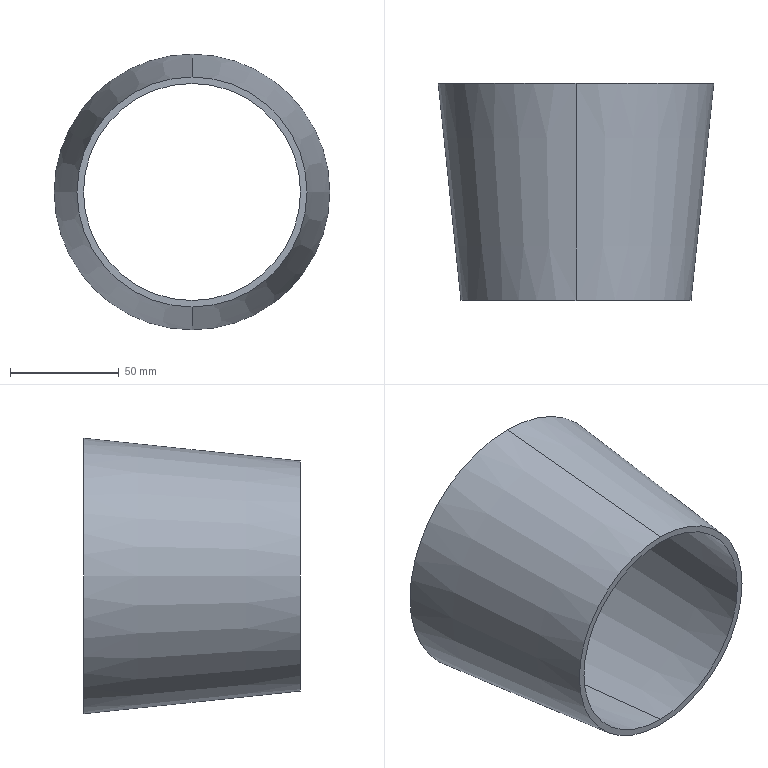Part | STEP file | getao1 | 1 solid | 6 faces | box 126.7 x 99.651 x 126.7 mm | volume 106341 mm3 | cone 4 | plane 2
STEP:
#1=CARTESIAN_POINT('',(0.,-164.318,-49.876));
#2=VERTEX_POINT('',#1);
#3=CARTESIAN_POINT('',(0.,-164.318,49.876));
#4=VERTEX_POINT('',#3);
#5=CARTESIAN_POINT('',(0.,-164.318,0.));
#6=DIRECTION('',(0.,1.,0.));
#7=DIRECTION('',(0.,0.,1.));
#8=AXIS2_PLACEMENT_3D('',#5,#6,#7);
#9=CIRCLE('',#8,49.876);
#10=EDGE_CURVE('',#2,#4,#9,.T.);
#11=ORIENTED_EDGE('',*,*,#10,.F.);
#12=CARTESIAN_POINT('',(0.,-64.667,-60.35));
#13=VERTEX_POINT('',#12);
#14=CARTESIAN_POINT('',(0.,-64.667,-60.35));
#15=DIRECTION('',(0.,0.9945,-0.1045));
#16=VECTOR('',#15,1000.);
#17=LINE('',#14,#16);
#18=EDGE_CURVE('',#2,#13,#17,.T.);
#19=ORIENTED_EDGE('',*,*,#18,.T.);
#20=CARTESIAN_POINT('',(0.,-64.667,60.35));
#21=VERTEX_POINT('',#20);
#22=CARTESIAN_POINT('',(0.,-64.667,0.));
#23=DIRECTION('',(0.,1.,0.));
#24=DIRECTION('',(0.,0.,1.));
#25=AXIS2_PLACEMENT_3D('',#22,#23,#24);
#26=CIRCLE('',#25,60.35);
#27=EDGE_CURVE('',#13,#21,#26,.T.);
#28=ORIENTED_EDGE('',*,*,#27,.T.);
#29=CARTESIAN_POINT('',(0.,-64.667,60.35));
#30=DIRECTION('',(0.,0.9945,0.1045));
#31=VECTOR('',#30,1000.);
#32=LINE('',#29,#31);
#33=EDGE_CURVE('',#4,#21,#32,.T.);
#34=ORIENTED_EDGE('',*,*,#33,.F.);
#35=EDGE_LOOP('',(#11,#19,#28,#34));
#36=FACE_OUTER_BOUND('',#35,.T.);
#37=CARTESIAN_POINT('',(0.,-64.667,0.));
#38=DIRECTION('',(0.,1.,0.));
#39=DIRECTION('',(0.,0.,1.));
#40=AXIS2_PLACEMENT_3D('',#37,#38,#39);
#41=CONICAL_SURFACE('',#40,60.35,0.1047);
#42=ADVANCED_FACE('',(#36),#41,.F.);
#43=CARTESIAN_POINT('',(0.,-164.318,52.876));
#44=VERTEX_POINT('',#43);
#45=CARTESIAN_POINT('',(0.,-164.318,-52.876));
#46=VERTEX_POINT('',#45);
#47=CARTESIAN_POINT('',(0.,-164.318,0.));
#48=DIRECTION('',(0.,1.,0.));
#49=DIRECTION('',(0.,0.,1.));
#50=AXIS2_PLACEMENT_3D('',#47,#48,#49);
#51=CIRCLE('',#50,52.876);
#52=EDGE_CURVE('',#44,#46,#51,.T.);
#53=ORIENTED_EDGE('',*,*,#52,.T.);
#54=CARTESIAN_POINT('',(0.,-64.667,-63.35));
#55=VERTEX_POINT('',#54);
#56=CARTESIAN_POINT('',(0.,-164.318,-52.876));
#57=DIRECTION('',(0.,0.9945,-0.1045));
#58=VECTOR('',#57,1000.);
#59=LINE('',#56,#58);
#60=EDGE_CURVE('',#46,#55,#59,.T.);
#61=ORIENTED_EDGE('',*,*,#60,.T.);
#62=CARTESIAN_POINT('',(0.,-64.667,63.35));
#63=VERTEX_POINT('',#62);
#64=CARTESIAN_POINT('',(0.,-64.667,0.));
#65=DIRECTION('',(0.,1.,0.));
#66=DIRECTION('',(0.,0.,1.));
#67=AXIS2_PLACEMENT_3D('',#64,#65,#66);
#68=CIRCLE('',#67,63.35);
#69=EDGE_CURVE('',#63,#55,#68,.T.);
#70=ORIENTED_EDGE('',*,*,#69,.F.);
#71=CARTESIAN_POINT('',(0.,-164.318,52.876));
#72=DIRECTION('',(0.,0.9945,0.1045));
#73=VECTOR('',#72,1000.);
#74=LINE('',#71,#73);
#75=EDGE_CURVE('',#44,#63,#74,.T.);
#76=ORIENTED_EDGE('',*,*,#75,.F.);
#77=EDGE_LOOP('',(#53,#61,#70,#76));
#78=FACE_OUTER_BOUND('',#77,.T.);
#79=CARTESIAN_POINT('',(0.,-164.318,0.));
#80=DIRECTION('',(0.,1.,0.));
#81=DIRECTION('',(0.,0.,1.));
#82=AXIS2_PLACEMENT_3D('',#79,#80,#81);
#83=CONICAL_SURFACE('',#82,52.876,0.1047);
#84=ADVANCED_FACE('',(#78),#83,.T.);
#85=CARTESIAN_POINT('',(0.,-64.667,0.));
#86=DIRECTION('',(0.,1.,0.));
#87=DIRECTION('',(0.,0.,1.));
#88=AXIS2_PLACEMENT_3D('',#85,#86,#87);
#89=CIRCLE('',#88,60.35);
#90=EDGE_CURVE('',#21,#13,#89,.T.);
#91=ORIENTED_EDGE('',*,*,#90,.F.);
#92=ORIENTED_EDGE('',*,*,#27,.F.);
#93=EDGE_LOOP('',(#91,#92));
#94=FACE_BOUND('',#93,.T.);
#95=ORIENTED_EDGE('',*,*,#69,.T.);
#96=CARTESIAN_POINT('',(0.,-64.667,0.));
#97=DIRECTION('',(0.,1.,0.));
#98=DIRECTION('',(0.,0.,1.));
#99=AXIS2_PLACEMENT_3D('',#96,#97,#98);
#100=CIRCLE('',#99,63.35);
#101=EDGE_CURVE('',#55,#63,#100,.T.);
#102=ORIENTED_EDGE('',*,*,#101,.T.);
#103=EDGE_LOOP('',(#95,#102));
#104=FACE_OUTER_BOUND('',#103,.T.);
#105=CARTESIAN_POINT('',(60.35,-64.667,0.));
#106=DIRECTION('',(0.,-1.,0.));
#107=DIRECTION('',(0.,0.,-1.));
#108=AXIS2_PLACEMENT_3D('',#105,#106,#107);
#109=PLANE('',#108);
#110=ADVANCED_FACE('',(#94,#104),#109,.F.);
#111=ORIENTED_EDGE('',*,*,#60,.F.);
#112=CARTESIAN_POINT('',(0.,-164.318,0.));
#113=DIRECTION('',(0.,1.,0.));
#114=DIRECTION('',(0.,0.,1.));
#115=AXIS2_PLACEMENT_3D('',#112,#113,#114);
#116=CIRCLE('',#115,52.876);
#117=EDGE_CURVE('',#46,#44,#116,.T.);
#118=ORIENTED_EDGE('',*,*,#117,.T.);
#119=ORIENTED_EDGE('',*,*,#75,.T.);
#120=ORIENTED_EDGE('',*,*,#101,.F.);
#121=EDGE_LOOP('',(#111,#118,#119,#120));
#122=FACE_OUTER_BOUND('',#121,.T.);
#123=CARTESIAN_POINT('',(0.,-164.318,0.));
#124=DIRECTION('',(0.,1.,0.));
#125=DIRECTION('',(0.,0.,1.));
#126=AXIS2_PLACEMENT_3D('',#123,#124,#125);
#127=CONICAL_SURFACE('',#126,52.876,0.1047);
#128=ADVANCED_FACE('',(#122),#127,.T.);
#129=ORIENTED_EDGE('',*,*,#52,.F.);
#130=ORIENTED_EDGE('',*,*,#117,.F.);
#131=EDGE_LOOP('',(#129,#130));
#132=FACE_OUTER_BOUND('',#131,.T.);
#133=CARTESIAN_POINT('',(0.,-164.318,0.));
#134=DIRECTION('',(0.,1.,0.));
#135=DIRECTION('',(0.,0.,1.));
#136=AXIS2_PLACEMENT_3D('',#133,#134,#135);
#137=CIRCLE('',#136,49.876);
#138=EDGE_CURVE('',#4,#2,#137,.T.);
#139=ORIENTED_EDGE('',*,*,#138,.T.);
#140=ORIENTED_EDGE('',*,*,#10,.T.);
#141=EDGE_LOOP('',(#139,#140));
#142=FACE_BOUND('',#141,.T.);
#143=CARTESIAN_POINT('',(49.876,-164.318,0.));
#144=DIRECTION('',(0.,1.,0.));
#145=DIRECTION('',(0.,0.,1.));
#146=AXIS2_PLACEMENT_3D('',#143,#144,#145);
#147=PLANE('',#146);
#148=ADVANCED_FACE('',(#132,#142),#147,.F.);
#149=ORIENTED_EDGE('',*,*,#18,.F.);
#150=ORIENTED_EDGE('',*,*,#138,.F.);
#151=ORIENTED_EDGE('',*,*,#33,.T.);
#152=ORIENTED_EDGE('',*,*,#90,.T.);
#153=EDGE_LOOP('',(#149,#150,#151,#152));
#154=FACE_OUTER_BOUND('',#153,.T.);
#155=CARTESIAN_POINT('',(0.,-64.667,0.));
#156=DIRECTION('',(0.,1.,0.));
#157=DIRECTION('',(0.,0.,1.));
#158=AXIS2_PLACEMENT_3D('',#155,#156,#157);
#159=CONICAL_SURFACE('',#158,60.35,0.1047);
#160=ADVANCED_FACE('',(#154),#159,.F.);
#161=CLOSED_SHELL('',(#42,#84,#110,#128,#148,#160));
#162=MANIFOLD_SOLID_BREP('',#161);
#163=CARTESIAN_POINT('',(0.,0.,0.));
#164=DIRECTION('',(0.,0.,1.));
#165=DIRECTION('',(1.,0.,0.));
#166=AXIS2_PLACEMENT_3D('',#163,#164,#165);
#167=(LENGTH_UNIT()NAMED_UNIT(*)SI_UNIT(.MILLI.,.METRE.));
#168=UNCERTAINTY_MEASURE_WITH_UNIT(LENGTH_MEASURE(0.00001),#167,'','');
#169=(NAMED_UNIT(*)PLANE_ANGLE_UNIT()SI_UNIT($,.RADIAN.));
#170=(NAMED_UNIT(*)SI_UNIT($,.STERADIAN.)SOLID_ANGLE_UNIT());
#171=(GEOMETRIC_REPRESENTATION_CONTEXT(3)GLOBAL_UNCERTAINTY_ASSIGNED_CONTEXT((#168))GLOBAL_UNIT_ASSIGNED_CONTEXT((#167,#169,#170))REPRESENTATION_CONTEXT('',''));
#172=ADVANCED_BREP_SHAPE_REPRESENTATION('',(#162,#166),#171);